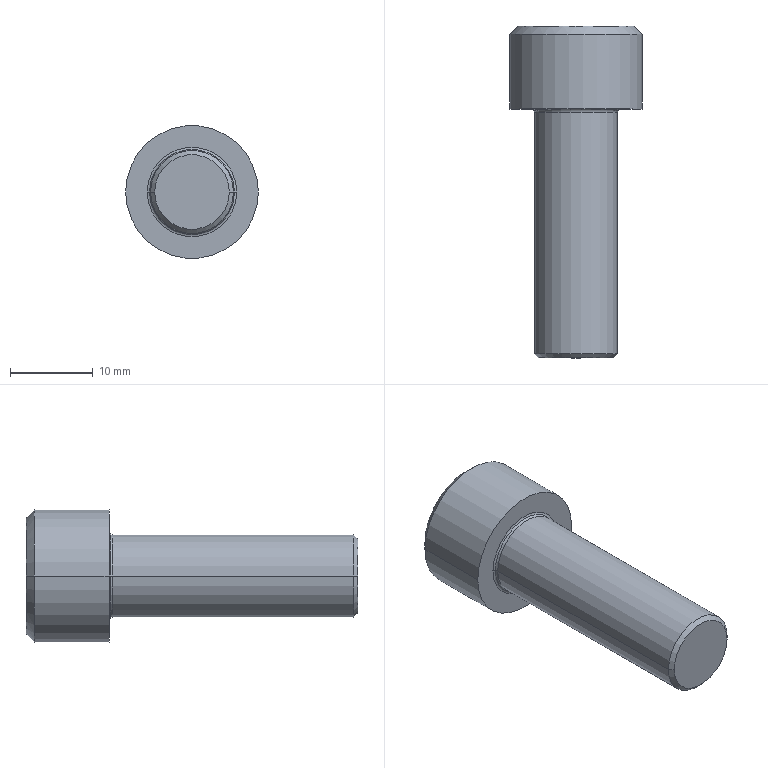Part | Creo | 1 solid | 23 faces | box 16 x 40 x 16 mm | volume 4005 mm3 | plane 9 | cone 6 | cylinder 4 | torus 4 | commonest cylinder face diameters 10 x2 16 x2
STEP:
#1=CARTESIAN_POINT('',(0.,0.,0.));
#2=DIRECTION('',(0.,0.,1.));
#3=DIRECTION('',(1.,0.,0.));
#4=AXIS2_PLACEMENT_3D('',#1,#2,#3);
#5=CARTESIAN_POINT('',(18.569,269.,-36.133));
#6=VERTEX_POINT('',#5);
#7=CARTESIAN_POINT('',(16.259,269.,-40.133));
#8=VERTEX_POINT('',#7);
#9=CARTESIAN_POINT('',(18.569,269.,-36.133));
#10=CARTESIAN_POINT('',(18.461,268.938,-36.32));
#11=CARTESIAN_POINT('',(18.245,268.826,-36.695));
#12=CARTESIAN_POINT('',(17.916,268.705,-37.265));
#13=CARTESIAN_POINT('',(17.583,268.64,-37.841));
#14=CARTESIAN_POINT('',(17.246,268.64,-38.424));
#15=CARTESIAN_POINT('',(16.913,268.704,-39.001));
#16=CARTESIAN_POINT('',(16.585,268.825,-39.57));
#17=CARTESIAN_POINT('',(16.368,268.938,-39.946));
#18=CARTESIAN_POINT('',(16.259,269.,-40.133));
#19=B_SPLINE_CURVE_WITH_KNOTS('',3,(#9,#10,#11,#12,#13,#14,#15,#16,#17,#18),.UNSPECIFIED.,.F.,.F.,(4,1,1,1,1,1,1,4),(0.,0.1429,0.2857,0.4286,0.5714,0.7143,0.8571,1.),.UNSPECIFIED.);
#20=EDGE_CURVE('',#6,#8,#19,.T.);
#21=ORIENTED_EDGE('',*,*,#20,.F.);
#22=CARTESIAN_POINT('',(13.95,266.333,-36.133));
#23=VERTEX_POINT('',#22);
#24=CARTESIAN_POINT('',(13.95,266.333,-36.133));
#25=DIRECTION('',(0.866,0.5,0.));
#26=VECTOR('',#25,5.333);
#27=LINE('',#24,#26);
#28=EDGE_CURVE('',#23,#6,#27,.T.);
#29=ORIENTED_EDGE('',*,*,#28,.F.);
#30=CARTESIAN_POINT('',(9.331,269.,-36.133));
#31=VERTEX_POINT('',#30);
#32=CARTESIAN_POINT('',(13.95,266.333,-36.133));
#33=DIRECTION('',(-0.866,0.5,0.));
#34=VECTOR('',#33,5.333);
#35=LINE('',#32,#34);
#36=EDGE_CURVE('',#23,#31,#35,.T.);
#37=ORIENTED_EDGE('',*,*,#36,.T.);
#38=CARTESIAN_POINT('',(11.641,269.,-40.133));
#39=VERTEX_POINT('',#38);
#40=CARTESIAN_POINT('',(11.641,269.,-40.133));
#41=CARTESIAN_POINT('',(11.533,268.938,-39.947));
#42=CARTESIAN_POINT('',(11.317,268.826,-39.572));
#43=CARTESIAN_POINT('',(10.988,268.705,-39.002));
#44=CARTESIAN_POINT('',(10.655,268.64,-38.426));
#45=CARTESIAN_POINT('',(10.318,268.64,-37.843));
#46=CARTESIAN_POINT('',(9.985,268.704,-37.266));
#47=CARTESIAN_POINT('',(9.656,268.825,-36.697));
#48=CARTESIAN_POINT('',(9.439,268.938,-36.321));
#49=CARTESIAN_POINT('',(9.331,269.,-36.133));
#50=B_SPLINE_CURVE_WITH_KNOTS('',3,(#40,#41,#42,#43,#44,#45,#46,#47,#48,#49),.UNSPECIFIED.,.F.,.F.,(4,1,1,1,1,1,1,4),(0.,0.1429,0.2857,0.4286,0.5714,0.7143,0.8571,1.),.UNSPECIFIED.);
#51=EDGE_CURVE('',#39,#31,#50,.T.);
#52=ORIENTED_EDGE('',*,*,#51,.F.);
#53=CARTESIAN_POINT('',(16.259,269.,-40.133));
#54=CARTESIAN_POINT('',(16.046,268.938,-40.133));
#55=CARTESIAN_POINT('',(15.615,268.827,-40.133));
#56=CARTESIAN_POINT('',(14.954,268.705,-40.133));
#57=CARTESIAN_POINT('',(14.285,268.64,-40.133));
#58=CARTESIAN_POINT('',(13.617,268.64,-40.133));
#59=CARTESIAN_POINT('',(12.95,268.704,-40.133));
#60=CARTESIAN_POINT('',(12.288,268.826,-40.133));
#61=CARTESIAN_POINT('',(11.856,268.938,-40.133));
#62=CARTESIAN_POINT('',(11.641,269.,-40.133));
#63=B_SPLINE_CURVE_WITH_KNOTS('',3,(#53,#54,#55,#56,#57,#58,#59,#60,#61,#62),.UNSPECIFIED.,.F.,.F.,(4,1,1,1,1,1,1,4),(0.,0.1429,0.2857,0.4286,0.5714,0.7143,0.8571,1.),.UNSPECIFIED.);
#64=EDGE_CURVE('',#8,#39,#63,.T.);
#65=ORIENTED_EDGE('',*,*,#64,.F.);
#66=EDGE_LOOP('',(#21,#29,#37,#52,#65));
#67=FACE_OUTER_BOUND('',#66,.F.);
#68=CARTESIAN_POINT('',(13.95,267.693,-36.133));
#69=DIRECTION('',(0.,1.,0.));
#70=DIRECTION('',(1.,0.,0.));
#71=AXIS2_PLACEMENT_3D('',#68,#69,#70);
#72=CONICAL_SURFACE('',#71,2.356,60.);
#73=ADVANCED_FACE('',(#67),#72,.F.);
#74=CARTESIAN_POINT('',(16.259,274.,-40.133));
#75=VERTEX_POINT('',#74);
#76=CARTESIAN_POINT('',(18.569,274.,-36.133));
#77=VERTEX_POINT('',#76);
#78=CARTESIAN_POINT('',(16.259,274.,-40.133));
#79=DIRECTION('',(0.5,0.,0.866));
#80=VECTOR('',#79,4.619);
#81=LINE('',#78,#80);
#82=EDGE_CURVE('',#75,#77,#81,.T.);
#83=ORIENTED_EDGE('',*,*,#82,.T.);
#84=CARTESIAN_POINT('',(18.569,274.,-36.133));
#85=DIRECTION('',(0.,-1.,0.));
#86=VECTOR('',#85,5.);
#87=LINE('',#84,#86);
#88=EDGE_CURVE('',#77,#6,#87,.T.);
#89=ORIENTED_EDGE('',*,*,#88,.T.);
#90=ORIENTED_EDGE('',*,*,#20,.T.);
#91=CARTESIAN_POINT('',(16.259,274.,-40.133));
#92=DIRECTION('',(0.,-1.,0.));
#93=VECTOR('',#92,5.);
#94=LINE('',#91,#93);
#95=EDGE_CURVE('',#75,#8,#94,.T.);
#96=ORIENTED_EDGE('',*,*,#95,.F.);
#97=EDGE_LOOP('',(#83,#89,#90,#96));
#98=FACE_OUTER_BOUND('',#97,.F.);
#99=CARTESIAN_POINT('',(16.259,269.,-40.133));
#100=DIRECTION('',(-0.866,0.,0.5));
#101=DIRECTION('',(0.5,0.,0.866));
#102=AXIS2_PLACEMENT_3D('',#99,#100,#101);
#103=PLANE('',#102);
#104=ADVANCED_FACE('',(#98),#103,.T.);
#105=CARTESIAN_POINT('',(20.95,274.,-36.133));
#106=VERTEX_POINT('',#105);
#107=CARTESIAN_POINT('',(6.95,274.,-36.133));
#108=VERTEX_POINT('',#107);
#109=CARTESIAN_POINT('',(13.95,274.,-36.133));
#110=DIRECTION('',(0.,1.,0.));
#111=DIRECTION('',(1.,0.,0.));
#112=AXIS2_PLACEMENT_3D('',#109,#110,#111);
#113=CIRCLE('',#112,7.);
#114=EDGE_CURVE('',#106,#108,#113,.T.);
#115=ORIENTED_EDGE('',*,*,#114,.F.);
#116=CARTESIAN_POINT('',(13.95,274.,-36.133));
#117=DIRECTION('',(0.,1.,0.));
#118=DIRECTION('',(-1.,0.,0.));
#119=AXIS2_PLACEMENT_3D('',#116,#117,#118);
#120=CIRCLE('',#119,7.);
#121=EDGE_CURVE('',#108,#106,#120,.T.);
#122=ORIENTED_EDGE('',*,*,#121,.F.);
#123=EDGE_LOOP('',(#115,#122));
#124=FACE_OUTER_BOUND('',#123,.F.);
#125=CARTESIAN_POINT('',(16.259,274.,-32.133));
#126=VERTEX_POINT('',#125);
#127=CARTESIAN_POINT('',(18.569,274.,-36.133));
#128=DIRECTION('',(-0.5,0.,0.866));
#129=VECTOR('',#128,4.619);
#130=LINE('',#127,#129);
#131=EDGE_CURVE('',#77,#126,#130,.T.);
#132=ORIENTED_EDGE('',*,*,#131,.F.);
#133=ORIENTED_EDGE('',*,*,#82,.F.);
#134=CARTESIAN_POINT('',(11.641,274.,-40.133));
#135=VERTEX_POINT('',#134);
#136=CARTESIAN_POINT('',(16.259,274.,-40.133));
#137=DIRECTION('',(-1.,0.,0.));
#138=VECTOR('',#137,4.619);
#139=LINE('',#136,#138);
#140=EDGE_CURVE('',#75,#135,#139,.T.);
#141=ORIENTED_EDGE('',*,*,#140,.T.);
#142=CARTESIAN_POINT('',(9.331,274.,-36.133));
#143=VERTEX_POINT('',#142);
#144=CARTESIAN_POINT('',(9.331,274.,-36.133));
#145=DIRECTION('',(0.5,0.,-0.866));
#146=VECTOR('',#145,4.619);
#147=LINE('',#144,#146);
#148=EDGE_CURVE('',#143,#135,#147,.T.);
#149=ORIENTED_EDGE('',*,*,#148,.F.);
#150=CARTESIAN_POINT('',(11.641,274.,-32.133));
#151=VERTEX_POINT('',#150);
#152=CARTESIAN_POINT('',(11.641,274.,-32.133));
#153=DIRECTION('',(-0.5,0.,-0.866));
#154=VECTOR('',#153,4.619);
#155=LINE('',#152,#154);
#156=EDGE_CURVE('',#151,#143,#155,.T.);
#157=ORIENTED_EDGE('',*,*,#156,.F.);
#158=CARTESIAN_POINT('',(11.641,274.,-32.133));
#159=DIRECTION('',(1.,0.,0.));
#160=VECTOR('',#159,4.619);
#161=LINE('',#158,#160);
#162=EDGE_CURVE('',#151,#126,#161,.T.);
#163=ORIENTED_EDGE('',*,*,#162,.T.);
#164=EDGE_LOOP('',(#132,#133,#141,#149,#157,#163));
#165=FACE_BOUND('',#164,.F.);
#166=CARTESIAN_POINT('',(13.95,274.,-36.133));
#167=DIRECTION('',(0.,1.,0.));
#168=DIRECTION('',(1.,0.,0.));
#169=AXIS2_PLACEMENT_3D('',#166,#167,#168);
#170=PLANE('',#169);
#171=ADVANCED_FACE('',(#124,#165),#170,.T.);
#172=CARTESIAN_POINT('',(21.95,273.,-36.133));
#173=VERTEX_POINT('',#172);
#174=CARTESIAN_POINT('',(5.95,273.,-36.133));
#175=VERTEX_POINT('',#174);
#176=CARTESIAN_POINT('',(13.95,273.,-36.133));
#177=DIRECTION('',(0.,1.,0.));
#178=DIRECTION('',(1.,0.,0.));
#179=AXIS2_PLACEMENT_3D('',#176,#177,#178);
#180=CIRCLE('',#179,8.);
#181=EDGE_CURVE('',#173,#175,#180,.T.);
#182=ORIENTED_EDGE('',*,*,#181,.F.);
#183=CARTESIAN_POINT('',(20.95,274.,-36.133));
#184=DIRECTION('',(0.7071,-0.7071,0.));
#185=VECTOR('',#184,1.414);
#186=LINE('',#183,#185);
#187=EDGE_CURVE('',#106,#173,#186,.T.);
#188=ORIENTED_EDGE('',*,*,#187,.F.);
#189=ORIENTED_EDGE('',*,*,#114,.T.);
#190=CARTESIAN_POINT('',(6.95,274.,-36.133));
#191=DIRECTION('',(-0.7071,-0.7071,0.));
#192=VECTOR('',#191,1.414);
#193=LINE('',#190,#192);
#194=EDGE_CURVE('',#108,#175,#193,.T.);
#195=ORIENTED_EDGE('',*,*,#194,.T.);
#196=EDGE_LOOP('',(#182,#188,#189,#195));
#197=FACE_OUTER_BOUND('',#196,.F.);
#198=CARTESIAN_POINT('',(13.95,273.5,-36.133));
#199=DIRECTION('',(0.,-1.,0.));
#200=DIRECTION('',(-1.,0.,0.));
#201=AXIS2_PLACEMENT_3D('',#198,#199,#200);
#202=CONICAL_SURFACE('',#201,7.5,45.);
#203=ADVANCED_FACE('',(#197),#202,.T.);
#204=ORIENTED_EDGE('',*,*,#181,.T.);
#205=CARTESIAN_POINT('',(5.95,264.,-36.133));
#206=VERTEX_POINT('',#205);
#207=CARTESIAN_POINT('',(5.95,264.,-36.133));
#208=DIRECTION('',(0.,1.,0.));
#209=VECTOR('',#208,9.);
#210=LINE('',#207,#209);
#211=EDGE_CURVE('',#206,#175,#210,.T.);
#212=ORIENTED_EDGE('',*,*,#211,.F.);
#213=CARTESIAN_POINT('',(21.95,264.,-36.133));
#214=VERTEX_POINT('',#213);
#215=CARTESIAN_POINT('',(13.95,264.,-36.133));
#216=DIRECTION('',(0.,-1.,0.));
#217=DIRECTION('',(-1.,0.,0.));
#218=AXIS2_PLACEMENT_3D('',#215,#216,#217);
#219=CIRCLE('',#218,8.);
#220=EDGE_CURVE('',#206,#214,#219,.T.);
#221=ORIENTED_EDGE('',*,*,#220,.T.);
#222=CARTESIAN_POINT('',(21.95,264.,-36.133));
#223=DIRECTION('',(0.,1.,0.));
#224=VECTOR('',#223,9.);
#225=LINE('',#222,#224);
#226=EDGE_CURVE('',#214,#173,#225,.T.);
#227=ORIENTED_EDGE('',*,*,#226,.T.);
#228=EDGE_LOOP('',(#204,#212,#221,#227));
#229=FACE_OUTER_BOUND('',#228,.F.);
#230=CARTESIAN_POINT('',(13.95,264.,-36.133));
#231=DIRECTION('',(0.,1.,0.));
#232=DIRECTION('',(1.,0.,0.));
#233=AXIS2_PLACEMENT_3D('',#230,#231,#232);
#234=CYLINDRICAL_SURFACE('',#233,8.);
#235=ADVANCED_FACE('',(#229),#234,.T.);
#236=CARTESIAN_POINT('',(13.95,273.,-36.133));
#237=DIRECTION('',(0.,1.,0.));
#238=DIRECTION('',(-1.,0.,0.));
#239=AXIS2_PLACEMENT_3D('',#236,#237,#238);
#240=CIRCLE('',#239,8.);
#241=EDGE_CURVE('',#175,#173,#240,.T.);
#242=ORIENTED_EDGE('',*,*,#241,.T.);
#243=ORIENTED_EDGE('',*,*,#226,.F.);
#244=CARTESIAN_POINT('',(13.95,264.,-36.133));
#245=DIRECTION('',(0.,-1.,0.));
#246=DIRECTION('',(1.,0.,0.));
#247=AXIS2_PLACEMENT_3D('',#244,#245,#246);
#248=CIRCLE('',#247,8.);
#249=EDGE_CURVE('',#214,#206,#248,.T.);
#250=ORIENTED_EDGE('',*,*,#249,.T.);
#251=ORIENTED_EDGE('',*,*,#211,.T.);
#252=EDGE_LOOP('',(#242,#243,#250,#251));
#253=FACE_OUTER_BOUND('',#252,.F.);
#254=CARTESIAN_POINT('',(13.95,264.,-36.133));
#255=DIRECTION('',(0.,1.,0.));
#256=DIRECTION('',(1.,0.,0.));
#257=AXIS2_PLACEMENT_3D('',#254,#255,#256);
#258=CYLINDRICAL_SURFACE('',#257,8.);
#259=ADVANCED_FACE('',(#253),#258,.T.);
#260=ORIENTED_EDGE('',*,*,#241,.F.);
#261=ORIENTED_EDGE('',*,*,#194,.F.);
#262=ORIENTED_EDGE('',*,*,#121,.T.);
#263=ORIENTED_EDGE('',*,*,#187,.T.);
#264=EDGE_LOOP('',(#260,#261,#262,#263));
#265=FACE_OUTER_BOUND('',#264,.F.);
#266=CARTESIAN_POINT('',(13.95,273.5,-36.133));
#267=DIRECTION('',(0.,-1.,0.));
#268=DIRECTION('',(-1.,0.,0.));
#269=AXIS2_PLACEMENT_3D('',#266,#267,#268);
#270=CONICAL_SURFACE('',#269,7.5,45.);
#271=ADVANCED_FACE('',(#265),#270,.T.);
#272=ORIENTED_EDGE('',*,*,#249,.F.);
#273=ORIENTED_EDGE('',*,*,#220,.F.);
#274=EDGE_LOOP('',(#272,#273));
#275=FACE_OUTER_BOUND('',#274,.F.);
#276=CARTESIAN_POINT('',(19.35,264.,-36.133));
#277=VERTEX_POINT('',#276);
#278=CARTESIAN_POINT('',(8.55,264.,-36.133));
#279=VERTEX_POINT('',#278);
#280=CARTESIAN_POINT('',(13.95,264.,-36.133));
#281=DIRECTION('',(0.,1.,0.));
#282=DIRECTION('',(1.,0.,0.));
#283=AXIS2_PLACEMENT_3D('',#280,#281,#282);
#284=CIRCLE('',#283,5.4);
#285=EDGE_CURVE('',#277,#279,#284,.T.);
#286=ORIENTED_EDGE('',*,*,#285,.F.);
#287=CARTESIAN_POINT('',(13.95,264.,-36.133));
#288=DIRECTION('',(0.,1.,0.));
#289=DIRECTION('',(-1.,0.,0.));
#290=AXIS2_PLACEMENT_3D('',#287,#288,#289);
#291=CIRCLE('',#290,5.4);
#292=EDGE_CURVE('',#279,#277,#291,.T.);
#293=ORIENTED_EDGE('',*,*,#292,.F.);
#294=EDGE_LOOP('',(#286,#293));
#295=FACE_BOUND('',#294,.F.);
#296=CARTESIAN_POINT('',(13.95,264.,-36.133));
#297=DIRECTION('',(0.,1.,0.));
#298=DIRECTION('',(1.,0.,0.));
#299=AXIS2_PLACEMENT_3D('',#296,#297,#298);
#300=PLANE('',#299);
#301=ADVANCED_FACE('',(#275,#295),#300,.F.);
#302=ORIENTED_EDGE('',*,*,#285,.T.);
#303=CARTESIAN_POINT('',(8.833,263.883,-36.133));
#304=VERTEX_POINT('',#303);
#305=CARTESIAN_POINT('',(8.55,263.6,-36.133));
#306=DIRECTION('',(0.,0.,-1.));
#307=DIRECTION('',(0.,1.,0.));
#308=AXIS2_PLACEMENT_3D('',#305,#306,#307);
#309=CIRCLE('',#308,0.4);
#310=EDGE_CURVE('',#279,#304,#309,.T.);
#311=ORIENTED_EDGE('',*,*,#310,.T.);
#312=CARTESIAN_POINT('',(19.067,263.883,-36.133));
#313=VERTEX_POINT('',#312);
#314=CARTESIAN_POINT('',(13.95,263.883,-36.133));
#315=DIRECTION('',(0.,1.,0.));
#316=DIRECTION('',(1.,0.,0.));
#317=AXIS2_PLACEMENT_3D('',#314,#315,#316);
#318=CIRCLE('',#317,5.117);
#319=EDGE_CURVE('',#313,#304,#318,.T.);
#320=ORIENTED_EDGE('',*,*,#319,.F.);
#321=CARTESIAN_POINT('',(19.35,263.6,-36.133));
#322=DIRECTION('',(0.,0.,1.));
#323=DIRECTION('',(0.,1.,0.));
#324=AXIS2_PLACEMENT_3D('',#321,#322,#323);
#325=CIRCLE('',#324,0.4);
#326=EDGE_CURVE('',#277,#313,#325,.T.);
#327=ORIENTED_EDGE('',*,*,#326,.F.);
#328=EDGE_LOOP('',(#302,#311,#320,#327));
#329=FACE_OUTER_BOUND('',#328,.F.);
#330=CARTESIAN_POINT('',(13.95,263.6,-36.133));
#331=DIRECTION('',(0.,1.,0.));
#332=DIRECTION('',(1.,0.,0.));
#333=AXIS2_PLACEMENT_3D('',#330,#331,#332);
#334=TOROIDAL_SURFACE('',#333,5.4,0.4);
#335=ADVANCED_FACE('',(#329),#334,.F.);
#336=ORIENTED_EDGE('',*,*,#292,.T.);
#337=ORIENTED_EDGE('',*,*,#326,.T.);
#338=CARTESIAN_POINT('',(13.95,263.883,-36.133));
#339=DIRECTION('',(0.,1.,0.));
#340=DIRECTION('',(-1.,0.,0.));
#341=AXIS2_PLACEMENT_3D('',#338,#339,#340);
#342=CIRCLE('',#341,5.117);
#343=EDGE_CURVE('',#304,#313,#342,.T.);
#344=ORIENTED_EDGE('',*,*,#343,.F.);
#345=ORIENTED_EDGE('',*,*,#310,.F.);
#346=EDGE_LOOP('',(#336,#337,#344,#345));
#347=FACE_OUTER_BOUND('',#346,.F.);
#348=CARTESIAN_POINT('',(13.95,263.6,-36.133));
#349=DIRECTION('',(0.,1.,0.));
#350=DIRECTION('',(1.,0.,0.));
#351=AXIS2_PLACEMENT_3D('',#348,#349,#350);
#352=TOROIDAL_SURFACE('',#351,5.4,0.4);
#353=ADVANCED_FACE('',(#347),#352,.F.);
#354=CARTESIAN_POINT('',(8.95,263.6,-36.133));
#355=VERTEX_POINT('',#354);
#356=CARTESIAN_POINT('',(18.95,263.6,-36.133));
#357=VERTEX_POINT('',#356);
#358=CARTESIAN_POINT('',(13.95,263.6,-36.133));
#359=DIRECTION('',(0.,1.,0.));
#360=DIRECTION('',(-1.,0.,0.));
#361=AXIS2_PLACEMENT_3D('',#358,#359,#360);
#362=CIRCLE('',#361,5.);
#363=EDGE_CURVE('',#355,#357,#362,.T.);
#364=ORIENTED_EDGE('',*,*,#363,.F.);
#365=CARTESIAN_POINT('',(8.55,263.6,-36.133));
#366=DIRECTION('',(0.,0.,-1.));
#367=DIRECTION('',(0.7071,0.7071,0.));
#368=AXIS2_PLACEMENT_3D('',#365,#366,#367);
#369=CIRCLE('',#368,0.4);
#370=EDGE_CURVE('',#304,#355,#369,.T.);
#371=ORIENTED_EDGE('',*,*,#370,.F.);
#372=ORIENTED_EDGE('',*,*,#343,.T.);
#373=CARTESIAN_POINT('',(19.35,263.6,-36.133));
#374=DIRECTION('',(0.,0.,1.));
#375=DIRECTION('',(-0.7071,0.7071,0.));
#376=AXIS2_PLACEMENT_3D('',#373,#374,#375);
#377=CIRCLE('',#376,0.4);
#378=EDGE_CURVE('',#313,#357,#377,.T.);
#379=ORIENTED_EDGE('',*,*,#378,.T.);
#380=EDGE_LOOP('',(#364,#371,#372,#379));
#381=FACE_OUTER_BOUND('',#380,.F.);
#382=CARTESIAN_POINT('',(13.95,263.6,-36.133));
#383=DIRECTION('',(0.,1.,0.));
#384=DIRECTION('',(1.,0.,0.));
#385=AXIS2_PLACEMENT_3D('',#382,#383,#384);
#386=TOROIDAL_SURFACE('',#385,5.4,0.4);
#387=ADVANCED_FACE('',(#381),#386,.F.);
#388=CARTESIAN_POINT('',(18.95,234.5,-36.133));
#389=VERTEX_POINT('',#388);
#390=CARTESIAN_POINT('',(8.95,234.5,-36.133));
#391=VERTEX_POINT('',#390);
#392=CARTESIAN_POINT('',(13.95,234.5,-36.133));
#393=DIRECTION('',(0.,-1.,0.));
#394=DIRECTION('',(1.,0.,0.));
#395=AXIS2_PLACEMENT_3D('',#392,#393,#394);
#396=CIRCLE('',#395,5.);
#397=EDGE_CURVE('',#389,#391,#396,.T.);
#398=ORIENTED_EDGE('',*,*,#397,.T.);
#399=CARTESIAN_POINT('',(8.95,234.5,-36.133));
#400=DIRECTION('',(0.,1.,0.));
#401=VECTOR('',#400,29.1);
#402=LINE('',#399,#401);
#403=EDGE_CURVE('',#391,#355,#402,.T.);
#404=ORIENTED_EDGE('',*,*,#403,.T.);
#405=ORIENTED_EDGE('',*,*,#363,.T.);
#406=CARTESIAN_POINT('',(18.95,234.5,-36.133));
#407=DIRECTION('',(0.,1.,0.));
#408=VECTOR('',#407,29.1);
#409=LINE('',#406,#408);
#410=EDGE_CURVE('',#389,#357,#409,.T.);
#411=ORIENTED_EDGE('',*,*,#410,.F.);
#412=EDGE_LOOP('',(#398,#404,#405,#411));
#413=FACE_OUTER_BOUND('',#412,.F.);
#414=CARTESIAN_POINT('',(13.95,234.,-36.133));
#415=DIRECTION('',(0.,1.,0.));
#416=DIRECTION('',(1.,0.,0.));
#417=AXIS2_PLACEMENT_3D('',#414,#415,#416);
#418=CYLINDRICAL_SURFACE('',#417,5.);
#419=ADVANCED_FACE('',(#413),#418,.T.);
#420=CARTESIAN_POINT('',(18.45,234.,-36.133));
#421=VERTEX_POINT('',#420);
#422=CARTESIAN_POINT('',(9.45,234.,-36.133));
#423=VERTEX_POINT('',#422);
#424=CARTESIAN_POINT('',(13.95,234.,-36.133));
#425=DIRECTION('',(0.,-1.,0.));
#426=DIRECTION('',(1.,0.,0.));
#427=AXIS2_PLACEMENT_3D('',#424,#425,#426);
#428=CIRCLE('',#427,4.5);
#429=EDGE_CURVE('',#421,#423,#428,.T.);
#430=ORIENTED_EDGE('',*,*,#429,.T.);
#431=CARTESIAN_POINT('',(9.45,234.,-36.133));
#432=DIRECTION('',(-0.7071,0.7071,0.));
#433=VECTOR('',#432,0.7071);
#434=LINE('',#431,#433);
#435=EDGE_CURVE('',#423,#391,#434,.T.);
#436=ORIENTED_EDGE('',*,*,#435,.T.);
#437=ORIENTED_EDGE('',*,*,#397,.F.);
#438=CARTESIAN_POINT('',(18.45,234.,-36.133));
#439=DIRECTION('',(0.7071,0.7071,0.));
#440=VECTOR('',#439,0.7071);
#441=LINE('',#438,#440);
#442=EDGE_CURVE('',#421,#389,#441,.T.);
#443=ORIENTED_EDGE('',*,*,#442,.F.);
#444=EDGE_LOOP('',(#430,#436,#437,#443));
#445=FACE_OUTER_BOUND('',#444,.F.);
#446=CARTESIAN_POINT('',(13.95,234.25,-36.133));
#447=DIRECTION('',(0.,1.,0.));
#448=DIRECTION('',(1.,0.,0.));
#449=AXIS2_PLACEMENT_3D('',#446,#447,#448);
#450=CONICAL_SURFACE('',#449,4.75,45.);
#451=ADVANCED_FACE('',(#445),#450,.T.);
#452=ORIENTED_EDGE('',*,*,#429,.F.);
#453=CARTESIAN_POINT('',(13.95,234.,-36.133));
#454=DIRECTION('',(0.,-1.,0.));
#455=DIRECTION('',(-1.,0.,0.));
#456=AXIS2_PLACEMENT_3D('',#453,#454,#455);
#457=CIRCLE('',#456,4.5);
#458=EDGE_CURVE('',#423,#421,#457,.T.);
#459=ORIENTED_EDGE('',*,*,#458,.F.);
#460=EDGE_LOOP('',(#452,#459));
#461=FACE_OUTER_BOUND('',#460,.F.);
#462=CARTESIAN_POINT('',(13.95,234.,-36.133));
#463=DIRECTION('',(0.,1.,0.));
#464=DIRECTION('',(1.,0.,0.));
#465=AXIS2_PLACEMENT_3D('',#462,#463,#464);
#466=PLANE('',#465);
#467=ADVANCED_FACE('',(#461),#466,.F.);
#468=ORIENTED_EDGE('',*,*,#458,.T.);
#469=ORIENTED_EDGE('',*,*,#442,.T.);
#470=CARTESIAN_POINT('',(13.95,234.5,-36.133));
#471=DIRECTION('',(0.,-1.,0.));
#472=DIRECTION('',(-1.,0.,0.));
#473=AXIS2_PLACEMENT_3D('',#470,#471,#472);
#474=CIRCLE('',#473,5.);
#475=EDGE_CURVE('',#391,#389,#474,.T.);
#476=ORIENTED_EDGE('',*,*,#475,.F.);
#477=ORIENTED_EDGE('',*,*,#435,.F.);
#478=EDGE_LOOP('',(#468,#469,#476,#477));
#479=FACE_OUTER_BOUND('',#478,.F.);
#480=CARTESIAN_POINT('',(13.95,234.25,-36.133));
#481=DIRECTION('',(0.,1.,0.));
#482=DIRECTION('',(1.,0.,0.));
#483=AXIS2_PLACEMENT_3D('',#480,#481,#482);
#484=CONICAL_SURFACE('',#483,4.75,45.);
#485=ADVANCED_FACE('',(#479),#484,.T.);
#486=ORIENTED_EDGE('',*,*,#475,.T.);
#487=ORIENTED_EDGE('',*,*,#410,.T.);
#488=CARTESIAN_POINT('',(13.95,263.6,-36.133));
#489=DIRECTION('',(0.,1.,0.));
#490=DIRECTION('',(1.,0.,0.));
#491=AXIS2_PLACEMENT_3D('',#488,#489,#490);
#492=CIRCLE('',#491,5.);
#493=EDGE_CURVE('',#357,#355,#492,.T.);
#494=ORIENTED_EDGE('',*,*,#493,.T.);
#495=ORIENTED_EDGE('',*,*,#403,.F.);
#496=EDGE_LOOP('',(#486,#487,#494,#495));
#497=FACE_OUTER_BOUND('',#496,.F.);
#498=CARTESIAN_POINT('',(13.95,234.,-36.133));
#499=DIRECTION('',(0.,1.,0.));
#500=DIRECTION('',(1.,0.,0.));
#501=AXIS2_PLACEMENT_3D('',#498,#499,#500);
#502=CYLINDRICAL_SURFACE('',#501,5.);
#503=ADVANCED_FACE('',(#497),#502,.T.);
#504=ORIENTED_EDGE('',*,*,#493,.F.);
#505=ORIENTED_EDGE('',*,*,#378,.F.);
#506=ORIENTED_EDGE('',*,*,#319,.T.);
#507=ORIENTED_EDGE('',*,*,#370,.T.);
#508=EDGE_LOOP('',(#504,#505,#506,#507));
#509=FACE_OUTER_BOUND('',#508,.F.);
#510=CARTESIAN_POINT('',(13.95,263.6,-36.133));
#511=DIRECTION('',(0.,1.,0.));
#512=DIRECTION('',(1.,0.,0.));
#513=AXIS2_PLACEMENT_3D('',#510,#511,#512);
#514=TOROIDAL_SURFACE('',#513,5.4,0.4);
#515=ADVANCED_FACE('',(#509),#514,.F.);
#516=ORIENTED_EDGE('',*,*,#131,.T.);
#517=CARTESIAN_POINT('',(16.259,269.,-32.133));
#518=VERTEX_POINT('',#517);
#519=CARTESIAN_POINT('',(16.259,274.,-32.133));
#520=DIRECTION('',(0.,-1.,0.));
#521=VECTOR('',#520,5.);
#522=LINE('',#519,#521);
#523=EDGE_CURVE('',#126,#518,#522,.T.);
#524=ORIENTED_EDGE('',*,*,#523,.T.);
#525=CARTESIAN_POINT('',(16.259,269.,-32.133));
#526=CARTESIAN_POINT('',(16.367,268.938,-32.32));
#527=CARTESIAN_POINT('',(16.583,268.826,-32.695));
#528=CARTESIAN_POINT('',(16.912,268.705,-33.265));
#529=CARTESIAN_POINT('',(17.245,268.64,-33.841));
#530=CARTESIAN_POINT('',(17.582,268.64,-34.424));
#531=CARTESIAN_POINT('',(17.915,268.704,-35.001));
#532=CARTESIAN_POINT('',(18.244,268.825,-35.57));
#533=CARTESIAN_POINT('',(18.461,268.938,-35.946));
#534=CARTESIAN_POINT('',(18.569,269.,-36.133));
#535=B_SPLINE_CURVE_WITH_KNOTS('',3,(#525,#526,#527,#528,#529,#530,#531,#532,#533,#534),.UNSPECIFIED.,.F.,.F.,(4,1,1,1,1,1,1,4),(0.,0.1429,0.2857,0.4286,0.5714,0.7143,0.8571,1.),.UNSPECIFIED.);
#536=EDGE_CURVE('',#518,#6,#535,.T.);
#537=ORIENTED_EDGE('',*,*,#536,.T.);
#538=ORIENTED_EDGE('',*,*,#88,.F.);
#539=EDGE_LOOP('',(#516,#524,#537,#538));
#540=FACE_OUTER_BOUND('',#539,.F.);
#541=CARTESIAN_POINT('',(18.569,269.,-36.133));
#542=DIRECTION('',(-0.866,0.,-0.5));
#543=DIRECTION('',(-0.5,0.,0.866));
#544=AXIS2_PLACEMENT_3D('',#541,#542,#543);
#545=PLANE('',#544);
#546=ADVANCED_FACE('',(#540),#545,.T.);
#547=ORIENTED_EDGE('',*,*,#162,.F.);
#548=CARTESIAN_POINT('',(11.641,269.,-32.133));
#549=VERTEX_POINT('',#548);
#550=CARTESIAN_POINT('',(11.641,274.,-32.133));
#551=DIRECTION('',(0.,-1.,0.));
#552=VECTOR('',#551,5.);
#553=LINE('',#550,#552);
#554=EDGE_CURVE('',#151,#549,#553,.T.);
#555=ORIENTED_EDGE('',*,*,#554,.T.);
#556=CARTESIAN_POINT('',(11.641,269.,-32.133));
#557=CARTESIAN_POINT('',(11.856,268.938,-32.133));
#558=CARTESIAN_POINT('',(12.288,268.826,-32.133));
#559=CARTESIAN_POINT('',(12.95,268.704,-32.133));
#560=CARTESIAN_POINT('',(13.617,268.64,-32.133));
#561=CARTESIAN_POINT('',(14.285,268.64,-32.133));
#562=CARTESIAN_POINT('',(14.954,268.705,-32.133));
#563=CARTESIAN_POINT('',(15.615,268.827,-32.133));
#564=CARTESIAN_POINT('',(16.046,268.938,-32.133));
#565=CARTESIAN_POINT('',(16.259,269.,-32.133));
#566=B_SPLINE_CURVE_WITH_KNOTS('',3,(#556,#557,#558,#559,#560,#561,#562,#563,#564,#565),.UNSPECIFIED.,.F.,.F.,(4,1,1,1,1,1,1,4),(0.,0.1429,0.2857,0.4286,0.5714,0.7143,0.8571,1.),.UNSPECIFIED.);
#567=EDGE_CURVE('',#549,#518,#566,.T.);
#568=ORIENTED_EDGE('',*,*,#567,.T.);
#569=ORIENTED_EDGE('',*,*,#523,.F.);
#570=EDGE_LOOP('',(#547,#555,#568,#569));
#571=FACE_OUTER_BOUND('',#570,.F.);
#572=CARTESIAN_POINT('',(16.259,269.,-32.133));
#573=DIRECTION('',(0.,0.,-1.));
#574=DIRECTION('',(0.,1.,0.));
#575=AXIS2_PLACEMENT_3D('',#572,#573,#574);
#576=PLANE('',#575);
#577=ADVANCED_FACE('',(#571),#576,.T.);
#578=ORIENTED_EDGE('',*,*,#156,.T.);
#579=CARTESIAN_POINT('',(9.331,274.,-36.133));
#580=DIRECTION('',(0.,-1.,0.));
#581=VECTOR('',#580,5.);
#582=LINE('',#579,#581);
#583=EDGE_CURVE('',#143,#31,#582,.T.);
#584=ORIENTED_EDGE('',*,*,#583,.T.);
#585=CARTESIAN_POINT('',(9.331,269.,-36.133));
#586=CARTESIAN_POINT('',(9.439,268.938,-35.946));
#587=CARTESIAN_POINT('',(9.656,268.825,-35.57));
#588=CARTESIAN_POINT('',(9.985,268.704,-35.001));
#589=CARTESIAN_POINT('',(10.318,268.64,-34.424));
#590=CARTESIAN_POINT('',(10.655,268.64,-33.841));
#591=CARTESIAN_POINT('',(10.988,268.705,-33.265));
#592=CARTESIAN_POINT('',(11.317,268.826,-32.695));
#593=CARTESIAN_POINT('',(11.533,268.938,-32.32));
#594=CARTESIAN_POINT('',(11.641,269.,-32.133));
#595=B_SPLINE_CURVE_WITH_KNOTS('',3,(#585,#586,#587,#588,#589,#590,#591,#592,#593,#594),.UNSPECIFIED.,.F.,.F.,(4,1,1,1,1,1,1,4),(0.,0.1429,0.2857,0.4286,0.5714,0.7143,0.8571,1.),.UNSPECIFIED.);
#596=EDGE_CURVE('',#31,#549,#595,.T.);
#597=ORIENTED_EDGE('',*,*,#596,.T.);
#598=ORIENTED_EDGE('',*,*,#554,.F.);
#599=EDGE_LOOP('',(#578,#584,#597,#598));
#600=FACE_OUTER_BOUND('',#599,.F.);
#601=CARTESIAN_POINT('',(11.641,269.,-32.133));
#602=DIRECTION('',(0.866,0.,-0.5));
#603=DIRECTION('',(-0.5,0.,-0.866));
#604=AXIS2_PLACEMENT_3D('',#601,#602,#603);
#605=PLANE('',#604);
#606=ADVANCED_FACE('',(#600),#605,.T.);
#607=ORIENTED_EDGE('',*,*,#148,.T.);
#608=CARTESIAN_POINT('',(11.641,274.,-40.133));
#609=DIRECTION('',(0.,-1.,0.));
#610=VECTOR('',#609,5.);
#611=LINE('',#608,#610);
#612=EDGE_CURVE('',#135,#39,#611,.T.);
#613=ORIENTED_EDGE('',*,*,#612,.T.);
#614=ORIENTED_EDGE('',*,*,#51,.T.);
#615=ORIENTED_EDGE('',*,*,#583,.F.);
#616=EDGE_LOOP('',(#607,#613,#614,#615));
#617=FACE_OUTER_BOUND('',#616,.F.);
#618=CARTESIAN_POINT('',(9.331,269.,-36.133));
#619=DIRECTION('',(0.866,0.,0.5));
#620=DIRECTION('',(0.5,0.,-0.866));
#621=AXIS2_PLACEMENT_3D('',#618,#619,#620);
#622=PLANE('',#621);
#623=ADVANCED_FACE('',(#617),#622,.T.);
#624=ORIENTED_EDGE('',*,*,#140,.F.);
#625=ORIENTED_EDGE('',*,*,#95,.T.);
#626=ORIENTED_EDGE('',*,*,#64,.T.);
#627=ORIENTED_EDGE('',*,*,#612,.F.);
#628=EDGE_LOOP('',(#624,#625,#626,#627));
#629=FACE_OUTER_BOUND('',#628,.F.);
#630=CARTESIAN_POINT('',(11.641,269.,-40.133));
#631=DIRECTION('',(0.,0.,1.));
#632=DIRECTION('',(0.,-1.,0.));
#633=AXIS2_PLACEMENT_3D('',#630,#631,#632);
#634=PLANE('',#633);
#635=ADVANCED_FACE('',(#629),#634,.T.);
#636=ORIENTED_EDGE('',*,*,#596,.F.);
#637=ORIENTED_EDGE('',*,*,#36,.F.);
#638=ORIENTED_EDGE('',*,*,#28,.T.);
#639=ORIENTED_EDGE('',*,*,#536,.F.);
#640=ORIENTED_EDGE('',*,*,#567,.F.);
#641=EDGE_LOOP('',(#636,#637,#638,#639,#640));
#642=FACE_OUTER_BOUND('',#641,.F.);
#643=CARTESIAN_POINT('',(13.95,267.693,-36.133));
#644=DIRECTION('',(0.,1.,0.));
#645=DIRECTION('',(1.,0.,0.));
#646=AXIS2_PLACEMENT_3D('',#643,#644,#645);
#647=CONICAL_SURFACE('',#646,2.356,60.);
#648=ADVANCED_FACE('',(#642),#647,.F.);
#649=CLOSED_SHELL('',(#73,#104,#171,#203,#235,#259,#271,#301,#335,#353,#387,#419,#451,#467,#485,#503,#515,#546,#577,#606,#623,#635,#648));
#650=MANIFOLD_SOLID_BREP('',#649);
#651=(LENGTH_UNIT()NAMED_UNIT(*)SI_UNIT(.MILLI.,.METRE.));
#652=UNCERTAINTY_MEASURE_WITH_UNIT(LENGTH_MEASURE(0.004595),#651,'','');
#653=(NAMED_UNIT(*)PLANE_ANGLE_UNIT()SI_UNIT($,.RADIAN.));
#654=PLANE_ANGLE_MEASURE_WITH_UNIT(PLANE_ANGLE_MEASURE(0.01745),#653);
#655=(CONVERSION_BASED_UNIT('DEGREE',#654)NAMED_UNIT(*)PLANE_ANGLE_UNIT());
#656=(NAMED_UNIT(*)SI_UNIT($,.STERADIAN.)SOLID_ANGLE_UNIT());
#657=(GEOMETRIC_REPRESENTATION_CONTEXT(3)GLOBAL_UNCERTAINTY_ASSIGNED_CONTEXT((#652))GLOBAL_UNIT_ASSIGNED_CONTEXT((#651,#655,#656))REPRESENTATION_CONTEXT('',''));
#658=ADVANCED_BREP_SHAPE_REPRESENTATION('',(#4,#650),#657);